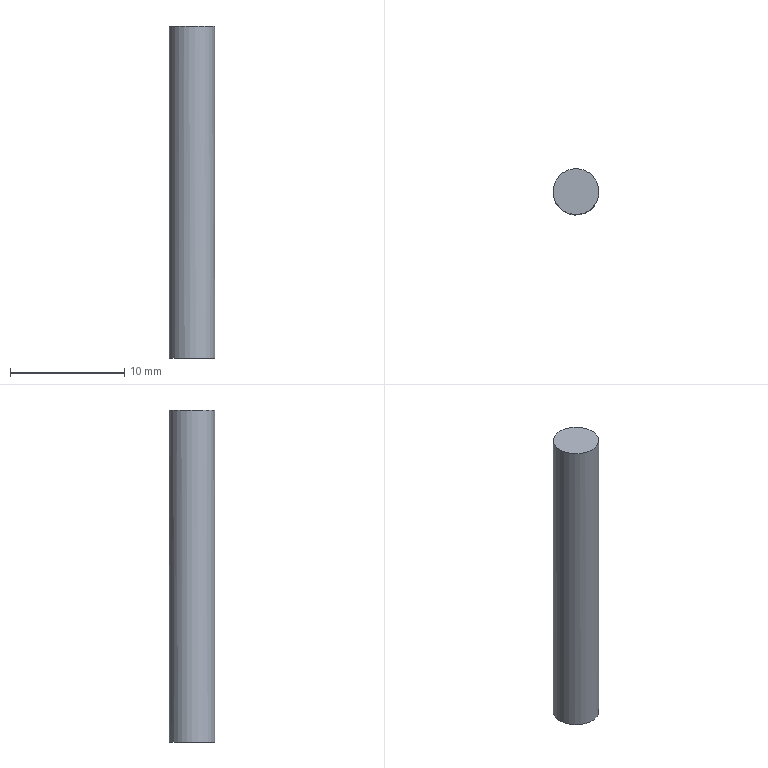Part | NX | features solid 2 | 1 solid | 3 faces | box 4 x 4 x 29 mm | volume 364.425 mm3 | plane 2 | cylinder 1 | commonest cylinder face diameters 4 x1
STEP:
#1=CARTESIAN_POINT('',(620.,-218.5,6.));
#2=VERTEX_POINT('',#1);
#3=CARTESIAN_POINT('',(620.,-220.5,6.));
#4=DIRECTION('',(0.,0.,-1.));
#5=DIRECTION('',(0.,1.,0.));
#6=AXIS2_PLACEMENT_3D('',#3,#4,#5);
#7=CIRCLE('',#6,2.);
#8=EDGE_CURVE('',#2,#2,#7,.T.);
#9=ORIENTED_EDGE('',*,*,#8,.T.);
#10=EDGE_LOOP('',(#9));
#11=FACE_BOUND('',#10,.T.);
#12=CARTESIAN_POINT('',(620.,-220.5,6.));
#13=DIRECTION('',(0.,0.,-1.));
#14=DIRECTION('',(0.,-1.,0.));
#15=AXIS2_PLACEMENT_3D('',#12,#13,#14);
#16=PLANE('',#15);
#17=ADVANCED_FACE('',(#11),#16,.T.);
#18=CARTESIAN_POINT('',(618.,-220.5,35.));
#19=VERTEX_POINT('',#18);
#20=CARTESIAN_POINT('',(620.,-220.5,35.));
#21=DIRECTION('',(0.,0.,-1.));
#22=DIRECTION('',(-1.,0.,0.));
#23=AXIS2_PLACEMENT_3D('',#20,#21,#22);
#24=CIRCLE('',#23,2.);
#25=EDGE_CURVE('',#19,#19,#24,.F.);
#26=ORIENTED_EDGE('',*,*,#25,.F.);
#27=EDGE_LOOP('',(#26));
#28=FACE_BOUND('',#27,.T.);
#29=ORIENTED_EDGE('',*,*,#8,.F.);
#30=EDGE_LOOP('',(#29));
#31=FACE_BOUND('',#30,.T.);
#32=CARTESIAN_POINT('',(620.,-220.5,36.));
#33=DIRECTION('',(0.,0.,-1.));
#34=DIRECTION('',(0.,-1.,0.));
#35=AXIS2_PLACEMENT_3D('',#32,#33,#34);
#36=CYLINDRICAL_SURFACE('',#35,2.);
#37=ADVANCED_FACE('',(#28,#31),#36,.T.);
#38=ORIENTED_EDGE('',*,*,#25,.T.);
#39=EDGE_LOOP('',(#38));
#40=FACE_BOUND('',#39,.T.);
#41=CARTESIAN_POINT('',(552.725,-187.,35.));
#42=DIRECTION('',(0.,0.,-1.));
#43=DIRECTION('',(0.,-1.,0.));
#44=AXIS2_PLACEMENT_3D('',#41,#42,#43);
#45=PLANE('',#44);
#46=ADVANCED_FACE('',(#40),#45,.F.);
#47=CLOSED_SHELL('',(#17,#37,#46));
#48=MANIFOLD_SOLID_BREP('',#47);
#49=(LENGTH_UNIT()NAMED_UNIT(*)SI_UNIT(.MILLI.,.METRE.));
#50=UNCERTAINTY_MEASURE_WITH_UNIT(LENGTH_MEASURE(0.00001),#49,'','');
#51=(NAMED_UNIT(*)PLANE_ANGLE_UNIT()SI_UNIT($,.RADIAN.));
#52=(NAMED_UNIT(*)SI_UNIT($,.STERADIAN.)SOLID_ANGLE_UNIT());
#53=(GEOMETRIC_REPRESENTATION_CONTEXT(3)GLOBAL_UNCERTAINTY_ASSIGNED_CONTEXT((#50))GLOBAL_UNIT_ASSIGNED_CONTEXT((#49,#51,#52))REPRESENTATION_CONTEXT('',''));
#54=ADVANCED_BREP_SHAPE_REPRESENTATION('',(#48),#53);